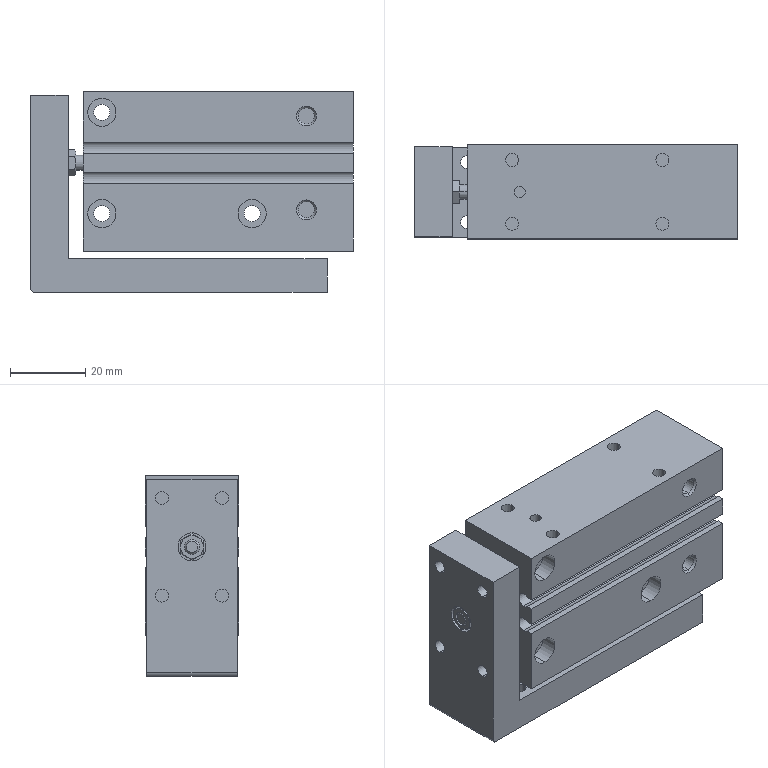Part | SolidWorks | features ICE 15, Chamfer 1, Extrusion 1, MirrorPattern 1, RevCut 1, Revolution 1 | 4 solids | 190 faces | box 86 x 25 x 53.5 mm | volume 94926 mm3 | cylinder 101 | plane 61 | cone 28 | commonest cylinder face diameters 3.44 x32 4 x20 4.3 x18 7.5 x18 4.2 x8 3 x2